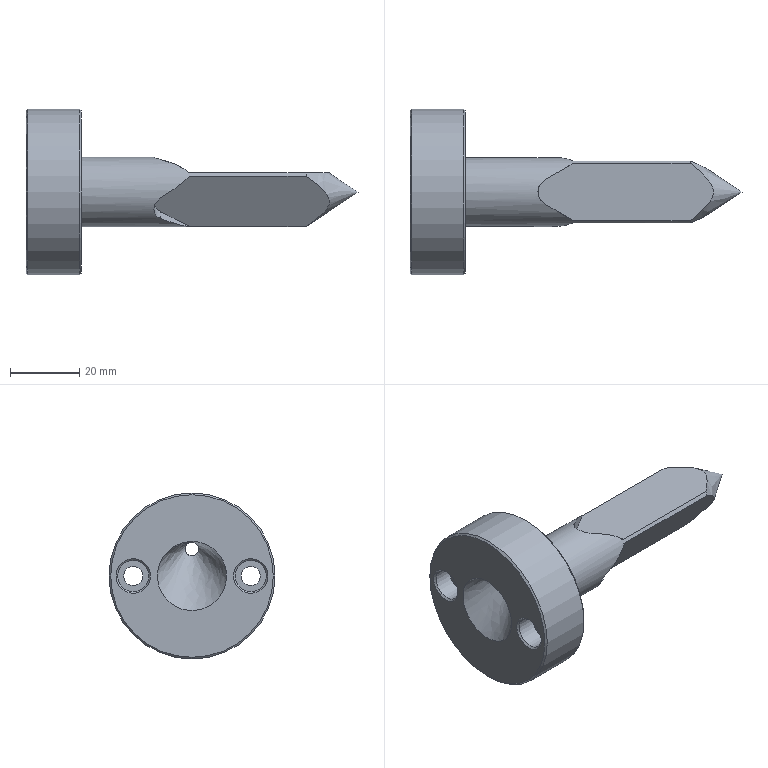Part | 1 solid | 31 faces | box 96 x 48 x 48 mm | volume 40853 mm3 | plane 13 | cylinder 11 | cone 5 | spline 2 | commonest cylinder face diameters 8 x3 4 x2 5.5 x2 9 x2 20 x1 48 x1